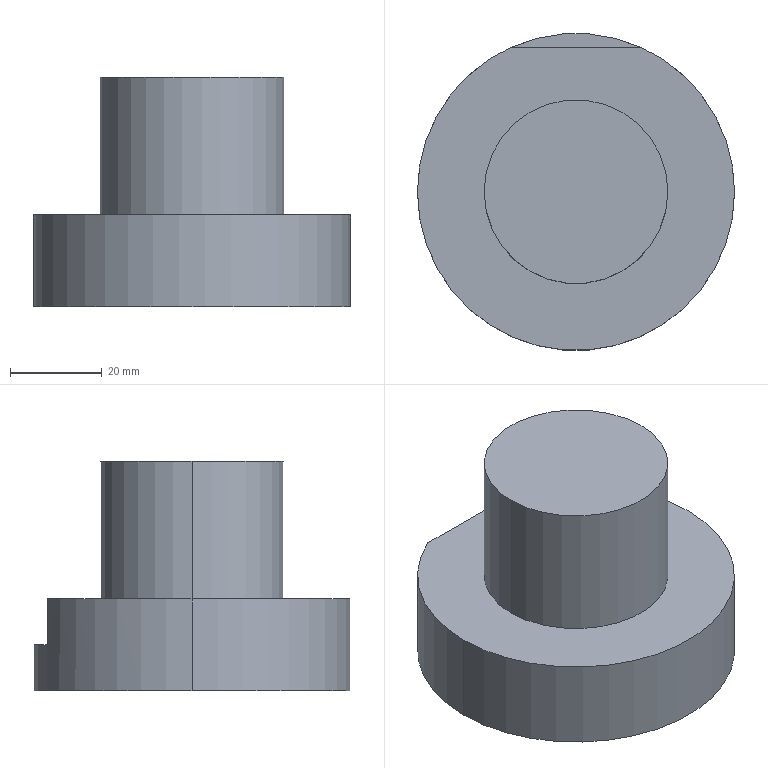Part | Mastercam | 1 solid | 9 faces | volume 111917 mm3 | plane 5 | cylinder 4 | commonest cylinder face diameters 40 x2 69 x2
STEP:
#1=CARTESIAN_POINT('',(0.,0.,0.));
#2=DIRECTION('',(0.,0.,1.));
#3=DIRECTION('',(1.,0.,0.));
#4=AXIS2_PLACEMENT_3D('',#1,#2,#3);
#5=CARTESIAN_POINT('',(-20.,0.,-30.));
#6=VERTEX_POINT('',#5);
#7=CARTESIAN_POINT('',(-20.,0.,0.));
#8=VERTEX_POINT('',#7);
#9=CARTESIAN_POINT('',(-20.,0.,-30.));
#10=DIRECTION('',(0.,0.,1.));
#11=VECTOR('',#10,1.);
#12=LINE('',#9,#11);
#13=EDGE_CURVE('',#6,#8,#12,.T.);
#14=ORIENTED_EDGE('',*,*,#13,.F.);
#15=CARTESIAN_POINT('',(20.,0.,-30.));
#16=VERTEX_POINT('',#15);
#17=CARTESIAN_POINT('',(0.,0.,-30.));
#18=DIRECTION('',(0.,0.,1.));
#19=DIRECTION('',(1.,0.,0.));
#20=AXIS2_PLACEMENT_3D('',#17,#18,#19);
#21=CIRCLE('',#20,20.);
#22=EDGE_CURVE('',#6,#16,#21,.T.);
#23=ORIENTED_EDGE('',*,*,#22,.T.);
#24=CARTESIAN_POINT('',(20.,0.,0.));
#25=VERTEX_POINT('',#24);
#26=CARTESIAN_POINT('',(20.,0.,-30.));
#27=DIRECTION('',(0.,0.,1.));
#28=VECTOR('',#27,1.);
#29=LINE('',#26,#28);
#30=EDGE_CURVE('',#16,#25,#29,.T.);
#31=ORIENTED_EDGE('',*,*,#30,.T.);
#32=CARTESIAN_POINT('',(0.,0.,0.));
#33=DIRECTION('',(0.,0.,1.));
#34=DIRECTION('',(1.,0.,0.));
#35=AXIS2_PLACEMENT_3D('',#32,#33,#34);
#36=CIRCLE('',#35,20.);
#37=EDGE_CURVE('',#8,#25,#36,.T.);
#38=ORIENTED_EDGE('',*,*,#37,.F.);
#39=EDGE_LOOP('',(#14,#23,#31,#38));
#40=FACE_OUTER_BOUND('',#39,.T.);
#41=CARTESIAN_POINT('',(0.,0.,-30.));
#42=DIRECTION('',(0.,0.,1.));
#43=DIRECTION('',(0.,1.,0.));
#44=AXIS2_PLACEMENT_3D('',#41,#42,#43);
#45=CYLINDRICAL_SURFACE('',#44,20.);
#46=ADVANCED_FACE('',(#40),#45,.T.);
#47=CARTESIAN_POINT('',(0.,0.,0.));
#48=DIRECTION('',(0.,0.,1.));
#49=DIRECTION('',(1.,0.,0.));
#50=AXIS2_PLACEMENT_3D('',#47,#48,#49);
#51=CIRCLE('',#50,20.);
#52=EDGE_CURVE('',#25,#8,#51,.T.);
#53=ORIENTED_EDGE('',*,*,#52,.T.);
#54=ORIENTED_EDGE('',*,*,#37,.T.);
#55=EDGE_LOOP('',(#53,#54));
#56=FACE_OUTER_BOUND('',#55,.T.);
#57=CARTESIAN_POINT('',(0.,0.,0.));
#58=DIRECTION('',(0.,0.,1.));
#59=DIRECTION('',(1.,0.,0.));
#60=AXIS2_PLACEMENT_3D('',#57,#58,#59);
#61=PLANE('',#60);
#62=ADVANCED_FACE('',(#56),#61,.T.);
#63=CARTESIAN_POINT('',(-34.5,0.,-50.));
#64=VERTEX_POINT('',#63);
#65=CARTESIAN_POINT('',(-34.5,0.,-30.));
#66=VERTEX_POINT('',#65);
#67=CARTESIAN_POINT('',(-34.5,0.,-50.));
#68=DIRECTION('',(0.,0.,1.));
#69=VECTOR('',#68,1.);
#70=LINE('',#67,#69);
#71=EDGE_CURVE('',#64,#66,#70,.T.);
#72=ORIENTED_EDGE('',*,*,#71,.F.);
#73=CARTESIAN_POINT('',(34.5,0.,-50.));
#74=VERTEX_POINT('',#73);
#75=CARTESIAN_POINT('',(0.,0.,-50.));
#76=DIRECTION('',(0.,0.,1.));
#77=DIRECTION('',(1.,0.,0.));
#78=AXIS2_PLACEMENT_3D('',#75,#76,#77);
#79=CIRCLE('',#78,34.5);
#80=EDGE_CURVE('',#64,#74,#79,.T.);
#81=ORIENTED_EDGE('',*,*,#80,.T.);
#82=CARTESIAN_POINT('',(34.5,0.,-30.));
#83=VERTEX_POINT('',#82);
#84=CARTESIAN_POINT('',(34.5,0.,-50.));
#85=DIRECTION('',(0.,0.,1.));
#86=VECTOR('',#85,1.);
#87=LINE('',#84,#86);
#88=EDGE_CURVE('',#74,#83,#87,.T.);
#89=ORIENTED_EDGE('',*,*,#88,.T.);
#90=CARTESIAN_POINT('',(0.,0.,-30.));
#91=DIRECTION('',(0.,0.,1.));
#92=DIRECTION('',(1.,0.,0.));
#93=AXIS2_PLACEMENT_3D('',#90,#91,#92);
#94=CIRCLE('',#93,34.5);
#95=EDGE_CURVE('',#66,#83,#94,.T.);
#96=ORIENTED_EDGE('',*,*,#95,.F.);
#97=EDGE_LOOP('',(#72,#81,#89,#96));
#98=FACE_OUTER_BOUND('',#97,.T.);
#99=CARTESIAN_POINT('',(0.,0.,-50.));
#100=DIRECTION('',(0.,0.,1.));
#101=DIRECTION('',(0.,1.,0.));
#102=AXIS2_PLACEMENT_3D('',#99,#100,#101);
#103=CYLINDRICAL_SURFACE('',#102,34.5);
#104=ADVANCED_FACE('',(#98),#103,.T.);
#105=ORIENTED_EDGE('',*,*,#80,.F.);
#106=CARTESIAN_POINT('',(0.,0.,-50.));
#107=DIRECTION('',(0.,0.,1.));
#108=DIRECTION('',(1.,0.,0.));
#109=AXIS2_PLACEMENT_3D('',#106,#107,#108);
#110=CIRCLE('',#109,34.5);
#111=EDGE_CURVE('',#74,#64,#110,.T.);
#112=ORIENTED_EDGE('',*,*,#111,.F.);
#113=EDGE_LOOP('',(#105,#112));
#114=FACE_OUTER_BOUND('',#113,.T.);
#115=CARTESIAN_POINT('',(0.,0.,-50.));
#116=DIRECTION('',(0.,0.,1.));
#117=DIRECTION('',(1.,0.,0.));
#118=AXIS2_PLACEMENT_3D('',#115,#116,#117);
#119=PLANE('',#118);
#120=ADVANCED_FACE('',(#114),#119,.F.);
#121=CARTESIAN_POINT('',(-14.071,31.5,-30.));
#122=VERTEX_POINT('',#121);
#123=CARTESIAN_POINT('',(14.071,31.5,-30.));
#124=VERTEX_POINT('',#123);
#125=CARTESIAN_POINT('',(-30.,31.5,-30.));
#126=DIRECTION('',(1.,0.,0.));
#127=VECTOR('',#126,1.);
#128=LINE('',#125,#127);
#129=EDGE_CURVE('',#122,#124,#128,.T.);
#130=ORIENTED_EDGE('',*,*,#129,.F.);
#131=CARTESIAN_POINT('',(0.,0.,-30.));
#132=DIRECTION('',(0.,0.,1.));
#133=DIRECTION('',(1.,0.,0.));
#134=AXIS2_PLACEMENT_3D('',#131,#132,#133);
#135=CIRCLE('',#134,34.5);
#136=EDGE_CURVE('',#122,#66,#135,.T.);
#137=ORIENTED_EDGE('',*,*,#136,.T.);
#138=ORIENTED_EDGE('',*,*,#95,.T.);
#139=CARTESIAN_POINT('',(0.,0.,-30.));
#140=DIRECTION('',(0.,0.,1.));
#141=DIRECTION('',(1.,0.,0.));
#142=AXIS2_PLACEMENT_3D('',#139,#140,#141);
#143=CIRCLE('',#142,34.5);
#144=EDGE_CURVE('',#83,#124,#143,.T.);
#145=ORIENTED_EDGE('',*,*,#144,.T.);
#146=EDGE_LOOP('',(#130,#137,#138,#145));
#147=FACE_OUTER_BOUND('',#146,.T.);
#148=ORIENTED_EDGE('',*,*,#22,.F.);
#149=CARTESIAN_POINT('',(0.,0.,-30.));
#150=DIRECTION('',(0.,0.,1.));
#151=DIRECTION('',(1.,0.,0.));
#152=AXIS2_PLACEMENT_3D('',#149,#150,#151);
#153=CIRCLE('',#152,20.);
#154=EDGE_CURVE('',#16,#6,#153,.T.);
#155=ORIENTED_EDGE('',*,*,#154,.F.);
#156=EDGE_LOOP('',(#148,#155));
#157=FACE_BOUND('',#156,.T.);
#158=CARTESIAN_POINT('',(0.,0.,-30.));
#159=DIRECTION('',(0.,0.,1.));
#160=DIRECTION('',(1.,0.,0.));
#161=AXIS2_PLACEMENT_3D('',#158,#159,#160);
#162=PLANE('',#161);
#163=ADVANCED_FACE('',(#147,#157),#162,.T.);
#164=CARTESIAN_POINT('',(14.071,31.5,-40.));
#165=VERTEX_POINT('',#164);
#166=CARTESIAN_POINT('',(-14.071,31.5,-40.));
#167=VERTEX_POINT('',#166);
#168=CARTESIAN_POINT('',(0.,0.,-40.));
#169=DIRECTION('',(0.,0.,1.));
#170=DIRECTION('',(-1.,0.,0.));
#171=AXIS2_PLACEMENT_3D('',#168,#169,#170);
#172=CIRCLE('',#171,34.5);
#173=EDGE_CURVE('',#165,#167,#172,.T.);
#174=ORIENTED_EDGE('',*,*,#173,.T.);
#175=CARTESIAN_POINT('',(-30.,31.5,-40.));
#176=DIRECTION('',(1.,0.,0.));
#177=VECTOR('',#176,1.);
#178=LINE('',#175,#177);
#179=EDGE_CURVE('',#167,#165,#178,.T.);
#180=ORIENTED_EDGE('',*,*,#179,.T.);
#181=EDGE_LOOP('',(#174,#180));
#182=FACE_OUTER_BOUND('',#181,.T.);
#183=CARTESIAN_POINT('',(-30.,51.5,-40.));
#184=DIRECTION('',(0.,0.,-1.));
#185=DIRECTION('',(-1.,0.,0.));
#186=AXIS2_PLACEMENT_3D('',#183,#184,#185);
#187=PLANE('',#186);
#188=ADVANCED_FACE('',(#182),#187,.F.);
#189=CARTESIAN_POINT('',(14.071,31.5,-50.));
#190=DIRECTION('',(0.,0.,-1.));
#191=VECTOR('',#190,1.);
#192=LINE('',#189,#191);
#193=EDGE_CURVE('',#124,#165,#192,.T.);
#194=ORIENTED_EDGE('',*,*,#193,.T.);
#195=ORIENTED_EDGE('',*,*,#179,.F.);
#196=CARTESIAN_POINT('',(-14.071,31.5,-50.));
#197=DIRECTION('',(0.,0.,1.));
#198=VECTOR('',#197,1.);
#199=LINE('',#196,#198);
#200=EDGE_CURVE('',#167,#122,#199,.T.);
#201=ORIENTED_EDGE('',*,*,#200,.T.);
#202=ORIENTED_EDGE('',*,*,#129,.T.);
#203=EDGE_LOOP('',(#194,#195,#201,#202));
#204=FACE_OUTER_BOUND('',#203,.T.);
#205=CARTESIAN_POINT('',(0.,31.5,0.));
#206=DIRECTION('',(0.,-1.,0.));
#207=DIRECTION('',(0.,0.,-1.));
#208=AXIS2_PLACEMENT_3D('',#205,#206,#207);
#209=PLANE('',#208);
#210=ADVANCED_FACE('',(#204),#209,.F.);
#211=ORIENTED_EDGE('',*,*,#13,.T.);
#212=ORIENTED_EDGE('',*,*,#52,.F.);
#213=ORIENTED_EDGE('',*,*,#30,.F.);
#214=ORIENTED_EDGE('',*,*,#154,.T.);
#215=EDGE_LOOP('',(#211,#212,#213,#214));
#216=FACE_OUTER_BOUND('',#215,.T.);
#217=CARTESIAN_POINT('',(0.,0.,-30.));
#218=DIRECTION('',(0.,0.,1.));
#219=DIRECTION('',(0.,-1.,0.));
#220=AXIS2_PLACEMENT_3D('',#217,#218,#219);
#221=CYLINDRICAL_SURFACE('',#220,20.);
#222=ADVANCED_FACE('',(#216),#221,.T.);
#223=ORIENTED_EDGE('',*,*,#71,.T.);
#224=ORIENTED_EDGE('',*,*,#136,.F.);
#225=ORIENTED_EDGE('',*,*,#200,.F.);
#226=ORIENTED_EDGE('',*,*,#173,.F.);
#227=ORIENTED_EDGE('',*,*,#193,.F.);
#228=ORIENTED_EDGE('',*,*,#144,.F.);
#229=ORIENTED_EDGE('',*,*,#88,.F.);
#230=ORIENTED_EDGE('',*,*,#111,.T.);
#231=EDGE_LOOP('',(#223,#224,#225,#226,#227,#228,#229,#230));
#232=FACE_OUTER_BOUND('',#231,.T.);
#233=CARTESIAN_POINT('',(0.,0.,-50.));
#234=DIRECTION('',(0.,0.,1.));
#235=DIRECTION('',(0.,-1.,0.));
#236=AXIS2_PLACEMENT_3D('',#233,#234,#235);
#237=CYLINDRICAL_SURFACE('',#236,34.5);
#238=ADVANCED_FACE('',(#232),#237,.T.);
#239=CLOSED_SHELL('',(#46,#62,#104,#120,#163,#188,#210,#222,#238));
#240=MANIFOLD_SOLID_BREP('',#239);
#241=CARTESIAN_POINT('',(6.96,18.75,-0.8));
#242=DIRECTION('',(-1.,0.,0.));
#243=VECTOR('',#242,1.);
#244=LINE('',#241,#243);
#245=TRIMMED_CURVE('',#244,(PARAMETER_VALUE(0.)),(PARAMETER_VALUE(13.919)),.T.,.PARAMETER.);
#246=CARTESIAN_POINT('',(10.121,17.25,-0.8));
#247=DIRECTION('',(-1.,0.,0.));
#248=VECTOR('',#247,1.);
#249=LINE('',#246,#248);
#250=TRIMMED_CURVE('',#249,(PARAMETER_VALUE(0.)),(PARAMETER_VALUE(20.242)),.T.,.PARAMETER.);
#251=CARTESIAN_POINT('',(12.326,15.75,-0.8));
#252=DIRECTION('',(-1.,0.,0.));
#253=VECTOR('',#252,1.);
#254=LINE('',#251,#253);
#255=TRIMMED_CURVE('',#254,(PARAMETER_VALUE(0.)),(PARAMETER_VALUE(24.653)),.T.,.PARAMETER.);
#256=CARTESIAN_POINT('',(14.033,14.25,-0.8));
#257=DIRECTION('',(-1.,0.,0.));
#258=VECTOR('',#257,1.);
#259=LINE('',#256,#258);
#260=TRIMMED_CURVE('',#259,(PARAMETER_VALUE(0.)),(PARAMETER_VALUE(28.067)),.T.,.PARAMETER.);
#261=CARTESIAN_POINT('',(-15.409,12.75,-0.8));
#262=DIRECTION('',(1.,0.,0.));
#263=VECTOR('',#262,1.);
#264=LINE('',#261,#263);
#265=TRIMMED_CURVE('',#264,(PARAMETER_VALUE(0.)),(PARAMETER_VALUE(30.818)),.T.,.PARAMETER.);
#266=CARTESIAN_POINT('',(-16.536,11.25,-0.8));
#267=DIRECTION('',(1.,0.,0.));
#268=VECTOR('',#267,1.);
#269=LINE('',#266,#268);
#270=TRIMMED_CURVE('',#269,(PARAMETER_VALUE(0.)),(PARAMETER_VALUE(33.072)),.T.,.PARAMETER.);
#271=CARTESIAN_POINT('',(-17.462,9.75,-0.8));
#272=DIRECTION('',(1.,0.,0.));
#273=VECTOR('',#272,1.);
#274=LINE('',#271,#273);
#275=TRIMMED_CURVE('',#274,(PARAMETER_VALUE(0.)),(PARAMETER_VALUE(34.925)),.T.,.PARAMETER.);
#276=CARTESIAN_POINT('',(18.219,8.25,-0.8));
#277=DIRECTION('',(-1.,0.,0.));
#278=VECTOR('',#277,1.);
#279=LINE('',#276,#278);
#280=TRIMMED_CURVE('',#279,(PARAMETER_VALUE(0.)),(PARAMETER_VALUE(36.438)),.T.,.PARAMETER.);
#281=CARTESIAN_POINT('',(-18.827,6.75,-0.8));
#282=DIRECTION('',(1.,0.,0.));
#283=VECTOR('',#282,1.);
#284=LINE('',#281,#283);
#285=TRIMMED_CURVE('',#284,(PARAMETER_VALUE(0.)),(PARAMETER_VALUE(37.653)),.T.,.PARAMETER.);
#286=CARTESIAN_POINT('',(19.299,5.25,-0.8));
#287=DIRECTION('',(-1.,0.,0.));
#288=VECTOR('',#287,1.);
#289=LINE('',#286,#288);
#290=TRIMMED_CURVE('',#289,(PARAMETER_VALUE(0.)),(PARAMETER_VALUE(38.597)),.T.,.PARAMETER.);
#291=CARTESIAN_POINT('',(-19.645,3.75,-0.8));
#292=DIRECTION('',(1.,0.,0.));
#293=VECTOR('',#292,1.);
#294=LINE('',#291,#293);
#295=TRIMMED_CURVE('',#294,(PARAMETER_VALUE(0.)),(PARAMETER_VALUE(39.291)),.T.,.PARAMETER.);
#296=CARTESIAN_POINT('',(19.873,2.25,-0.8));
#297=DIRECTION('',(-1.,0.,0.));
#298=VECTOR('',#297,1.);
#299=LINE('',#296,#298);
#300=TRIMMED_CURVE('',#299,(PARAMETER_VALUE(0.)),(PARAMETER_VALUE(39.746)),.T.,.PARAMETER.);
#301=CARTESIAN_POINT('',(-19.986,0.75,-0.8));
#302=DIRECTION('',(1.,0.,0.));
#303=VECTOR('',#302,1.);
#304=LINE('',#301,#303);
#305=TRIMMED_CURVE('',#304,(PARAMETER_VALUE(0.)),(PARAMETER_VALUE(39.972)),.T.,.PARAMETER.);
#306=CARTESIAN_POINT('',(19.986,-0.75,-0.8));
#307=DIRECTION('',(-1.,0.,0.));
#308=VECTOR('',#307,1.);
#309=LINE('',#306,#308);
#310=TRIMMED_CURVE('',#309,(PARAMETER_VALUE(0.)),(PARAMETER_VALUE(39.972)),.T.,.PARAMETER.);
#311=CARTESIAN_POINT('',(-19.873,-2.25,-0.8));
#312=DIRECTION('',(1.,0.,0.));
#313=VECTOR('',#312,1.);
#314=LINE('',#311,#313);
#315=TRIMMED_CURVE('',#314,(PARAMETER_VALUE(0.)),(PARAMETER_VALUE(39.746)),.T.,.PARAMETER.);
#316=CARTESIAN_POINT('',(19.645,-3.75,-0.8));
#317=DIRECTION('',(-1.,0.,0.));
#318=VECTOR('',#317,1.);
#319=LINE('',#316,#318);
#320=TRIMMED_CURVE('',#319,(PARAMETER_VALUE(0.)),(PARAMETER_VALUE(39.291)),.T.,.PARAMETER.);
#321=CARTESIAN_POINT('',(-19.299,-5.25,-0.8));
#322=DIRECTION('',(1.,0.,0.));
#323=VECTOR('',#322,1.);
#324=LINE('',#321,#323);
#325=TRIMMED_CURVE('',#324,(PARAMETER_VALUE(0.)),(PARAMETER_VALUE(38.597)),.T.,.PARAMETER.);
#326=CARTESIAN_POINT('',(18.827,-6.75,-0.8));
#327=DIRECTION('',(-1.,0.,0.));
#328=VECTOR('',#327,1.);
#329=LINE('',#326,#328);
#330=TRIMMED_CURVE('',#329,(PARAMETER_VALUE(0.)),(PARAMETER_VALUE(37.653)),.T.,.PARAMETER.);
#331=CARTESIAN_POINT('',(-18.219,-8.25,-0.8));
#332=DIRECTION('',(1.,0.,0.));
#333=VECTOR('',#332,1.);
#334=LINE('',#331,#333);
#335=TRIMMED_CURVE('',#334,(PARAMETER_VALUE(0.)),(PARAMETER_VALUE(36.438)),.T.,.PARAMETER.);
#336=CARTESIAN_POINT('',(-17.462,-9.75,-0.8));
#337=DIRECTION('',(1.,0.,0.));
#338=VECTOR('',#337,1.);
#339=LINE('',#336,#338);
#340=TRIMMED_CURVE('',#339,(PARAMETER_VALUE(0.)),(PARAMETER_VALUE(34.925)),.T.,.PARAMETER.);
#341=CARTESIAN_POINT('',(16.536,-11.25,-0.8));
#342=DIRECTION('',(-1.,0.,0.));
#343=VECTOR('',#342,1.);
#344=LINE('',#341,#343);
#345=TRIMMED_CURVE('',#344,(PARAMETER_VALUE(0.)),(PARAMETER_VALUE(33.072)),.T.,.PARAMETER.);
#346=CARTESIAN_POINT('',(-15.409,-12.75,-0.8));
#347=DIRECTION('',(1.,0.,0.));
#348=VECTOR('',#347,1.);
#349=LINE('',#346,#348);
#350=TRIMMED_CURVE('',#349,(PARAMETER_VALUE(0.)),(PARAMETER_VALUE(30.818)),.T.,.PARAMETER.);
#351=CARTESIAN_POINT('',(14.033,-14.25,-0.8));
#352=DIRECTION('',(-1.,0.,0.));
#353=VECTOR('',#352,1.);
#354=LINE('',#351,#353);
#355=TRIMMED_CURVE('',#354,(PARAMETER_VALUE(0.)),(PARAMETER_VALUE(28.067)),.T.,.PARAMETER.);
#356=CARTESIAN_POINT('',(-12.326,-15.75,-0.8));
#357=DIRECTION('',(1.,0.,0.));
#358=VECTOR('',#357,1.);
#359=LINE('',#356,#358);
#360=TRIMMED_CURVE('',#359,(PARAMETER_VALUE(0.)),(PARAMETER_VALUE(24.653)),.T.,.PARAMETER.);
#361=CARTESIAN_POINT('',(10.121,-17.25,-0.8));
#362=DIRECTION('',(-1.,0.,0.));
#363=VECTOR('',#362,1.);
#364=LINE('',#361,#363);
#365=TRIMMED_CURVE('',#364,(PARAMETER_VALUE(0.)),(PARAMETER_VALUE(20.242)),.T.,.PARAMETER.);
#366=CARTESIAN_POINT('',(-6.96,-18.75,-0.8));
#367=DIRECTION('',(1.,0.,0.));
#368=VECTOR('',#367,1.);
#369=LINE('',#366,#368);
#370=TRIMMED_CURVE('',#369,(PARAMETER_VALUE(0.)),(PARAMETER_VALUE(13.919)),.T.,.PARAMETER.);
#371=CARTESIAN_POINT('',(-6.96,-20.25,-0.8));
#372=DIRECTION('',(1.,0.,0.));
#373=VECTOR('',#372,1.);
#374=LINE('',#371,#373);
#375=TRIMMED_CURVE('',#374,(PARAMETER_VALUE(0.)),(PARAMETER_VALUE(13.919)),.T.,.PARAMETER.);
#376=CARTESIAN_POINT('',(-6.96,-21.75,0.));
#377=DIRECTION('',(1.,0.,0.));
#378=VECTOR('',#377,1.);
#379=LINE('',#376,#378);
#380=TRIMMED_CURVE('',#379,(PARAMETER_VALUE(0.)),(PARAMETER_VALUE(13.919)),.T.,.PARAMETER.);
#381=CARTESIAN_POINT('',(14.33,-18.816,26.702));
#382=DIRECTION('',(0.1045,0.9945,0.));
#383=DIRECTION('',(0.9945,-0.1045,0.));
#384=AXIS2_PLACEMENT_3D('',#381,#382,#383);
#385=CIRCLE('',#384,2.5);
#386=CARTESIAN_POINT('',(15.663,-6.133,26.702));
#387=DIRECTION('',(0.1045,0.9945,0.));
#388=DIRECTION('',(0.9945,-0.1045,0.));
#389=AXIS2_PLACEMENT_3D('',#386,#387,#388);
#390=CIRCLE('',#389,2.25);
#391=CARTESIAN_POINT('',(6.96,20.25,-0.8));
#392=DIRECTION('',(-1.,0.,0.));
#393=VECTOR('',#392,1.);
#394=LINE('',#391,#393);
#395=TRIMMED_CURVE('',#394,(PARAMETER_VALUE(0.)),(PARAMETER_VALUE(13.919)),.T.,.PARAMETER.);
#396=CARTESIAN_POINT('',(0.,0.,0.));
#397=DIRECTION('',(0.,0.,1.));
#398=DIRECTION('',(1.,0.,0.));
#399=AXIS2_PLACEMENT_3D('',#396,#397,#398);
#400=CIRCLE('',#399,20.);
#401=CARTESIAN_POINT('',(0.,27.4,-30.));
#402=DIRECTION('',(0.,0.,1.));
#403=DIRECTION('',(1.,0.,0.));
#404=AXIS2_PLACEMENT_3D('',#401,#402,#403);
#405=CIRCLE('',#404,2.5);
#406=CARTESIAN_POINT('',(-23.729,-13.7,-30.));
#407=DIRECTION('',(0.,0.,1.));
#408=DIRECTION('',(1.,0.,0.));
#409=AXIS2_PLACEMENT_3D('',#406,#407,#408);
#410=CIRCLE('',#409,2.5);
#411=CARTESIAN_POINT('',(23.729,-13.7,-30.));
#412=DIRECTION('',(0.,0.,1.));
#413=DIRECTION('',(1.,0.,0.));
#414=AXIS2_PLACEMENT_3D('',#411,#412,#413);
#415=CIRCLE('',#414,2.5);
#416=CARTESIAN_POINT('',(0.,0.,0.));
#417=DIRECTION('',(0.,0.,1.));
#418=DIRECTION('',(1.,0.,0.));
#419=AXIS2_PLACEMENT_3D('',#416,#417,#418);
#420=CIRCLE('',#419,16.);
#421=GEOMETRIC_CURVE_SET('',(#245,#250,#255,#260,#265,#270,#275,#280,#285,#290,#295,#300,#305,#310,#315,#320,#325,#330,#335,#340,#345,#350,#355,#360,#365,#370,#375,#380,#385,#390,#395,#400,#405,#410,#415,#420));
#422=(LENGTH_UNIT()NAMED_UNIT(*)SI_UNIT(.MILLI.,.METRE.));
#423=UNCERTAINTY_MEASURE_WITH_UNIT(LENGTH_MEASURE(0.005),#422,'','');
#424=(NAMED_UNIT(*)PLANE_ANGLE_UNIT()SI_UNIT($,.RADIAN.));
#425=(GEOMETRIC_REPRESENTATION_CONTEXT(3)GLOBAL_UNCERTAINTY_ASSIGNED_CONTEXT((#423))GLOBAL_UNIT_ASSIGNED_CONTEXT((#422,#424))REPRESENTATION_CONTEXT('',''));
#426=SHAPE_REPRESENTATION('',(#4,#240,#421),#425);